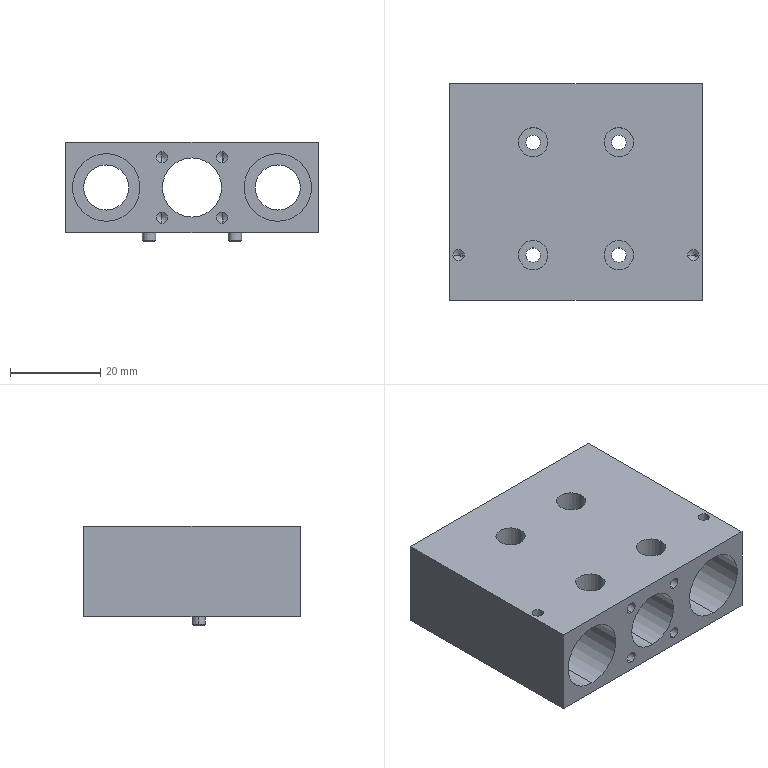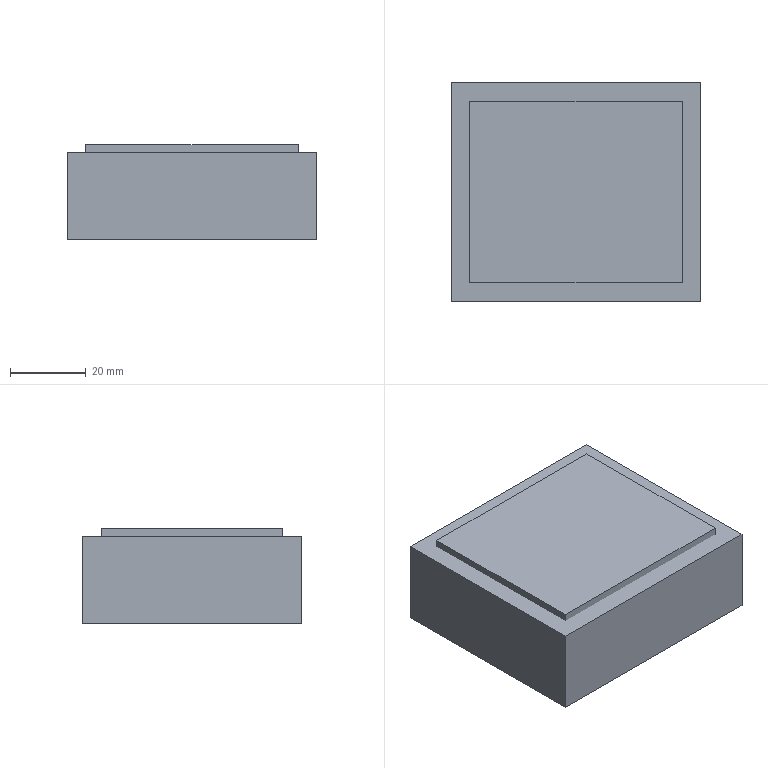CAM job | NX | 3+2 milling, drilling | part box 56 x 48 x 22 mm | stock box 66 x 58 x 25 mm
Tools:
number,name,description,diameter,corner_radius,flute_length,length,flutes
1,D63,Milling Tool-5 Parameters,63.0,0.0,50.0,75.0,2
7,D6A45,Milling Tool-5 Parameters,6.0,0.0,50.0,75.0,2
12,2.5ZT,Drilling Tool,2.5,0.0,35.0,50.0,2
13,3.2ZT,Drilling Tool,3.2,0.0,35.0,50.0,2
10,D10,Milling Tool-5 Parameters,10.0,0.0,50.0,75.0,2
4,D4,Milling Tool-5 Parameters,4.0,0.0,50.0,75.0,2
11,10.ZT,Drilling Tool,10.0,0.0,35.0,50.0,2
Operations:
program,operation,operation_type,tool,method,geometry_group,spindle_rpm,surface_speed,feed_per_tooth,feed_cut,feed_plunge,cut_length_mm,path_length_mm,cut_time_min,machine_time_min
1,FLOOR_WALL,VolumeBased25DMillingOperation,D63,METHOD,A,6500.0,1286.0,0.1154,1500.0,100.0,141.0,195.0,0.094,0.0994
1,DRILLING,Operation,D6A45,METHOD,A,5000.0,94.0,0.025,250.0,0.0,24.0,225.116,0.096,0.1161
1,DRILLING_COPY,Operation,2.5ZT,METHOD,A,2000.0,15.0,0.03,120.0,0.0,17.502,150.091,0.1459,0.1591
1,DRILLING_COPY_COPY,Operation,3.2ZT,METHOD,A,2000.0,15.0,0.03,120.0,0.0,101.846,342.705,0.8487,0.8728
1,ADAPTIVE_MILLING,CavityMilling,D10,METHOD,A,9500.0,298.0,0.1579,3000.0,1000.0,1490.014,1588.014,0.4987,0.5085
1,ZLEVEL_PROFILE,ZLevelMilling,D10,METHOD,A,9500.0,298.0,0.0789,1500.0,100.0,247.754,348.754,0.1652,0.1753
1,HOLE_MILLING,CylinderMilling,D4,METHOD,A,9500.0,119.0,0.0737,1400.0,100.0,479.653,807.053,0.3426,0.3753
1,PLANAR_MILL,PlanarMilling,D6A45,METHOD,A,9500.0,179.0,0.0658,1250.0,100.0,329.587,860.865,0.2637,0.3168
2,FLOOR_WALL_COPY,VolumeBased25DMillingOperation,D63,METHOD,B,6500.0,1286.0,0.1154,1500.0,100.0,405.0,819.001,0.27,0.3114
2,FLOOR_WALL_1,VolumeBased25DMillingOperation,D10,METHOD,B,9500.0,298.0,0.1316,2500.0,1000.0,1226.971,1307.507,0.5022,0.5102
2,FLOOR_WALL_1_COPY,VolumeBased25DMillingOperation,D10,METHOD,B,9500.0,298.0,0.0789,1500.0,1000.0,789.781,1111.681,0.5367,0.5689
2,PLANAR_MILL_COPY,PlanarMilling,D6A45,METHOD,B,9500.0,179.0,0.0658,1250.0,100.0,43.137,174.198,0.0345,0.0476
2,PLANAR_MILL_COPY_1,PlanarMilling,D6A45,METHOD,B,9500.0,179.0,0.0658,1250.0,100.0,266.484,660.617,0.2132,0.2526
3,DRILLING_COPY_1,Operation,D6A45,METHOD,C,5000.0,94.0,0.025,250.0,0.0,28.0,209.989,0.112,0.1302
3,DRILLING_COPY_COPY_1,Operation,2.5ZT,METHOD,C,2000.0,15.0,0.03,120.0,0.0,39.004,193.659,0.325,0.3405
3,DRILLING_COPY_COPY_1_COPY,Operation,10.ZT,METHOD,C,2000.0,15.0,0.03,120.0,0.0,166.513,456.379,1.388,1.417
3,HOLE_MILLING_1,CylinderMilling,D10,METHOD,C,6500.0,204.0,0.1154,1500.0,100.0,3085.831,3440.331,2.057,2.093
3,HOLE_MILLING_1_COPY,CylinderMilling,D10,METHOD,C,6500.0,204.0,0.0923,1200.0,100.0,465.546,712.546,0.388,0.4127
3,PLANAR_MILL_COPY_1_COPY,PlanarMilling,D6A45,METHOD,C,9500.0,179.0,0.0658,1250.0,100.0,343.361,863.869,0.2747,0.3267
3,刀补10,CylinderMilling,D10,METHOD,C,6500.0,204.0,0.0923,1200.0,100.0,153.486,260.986,0.1279,0.1387